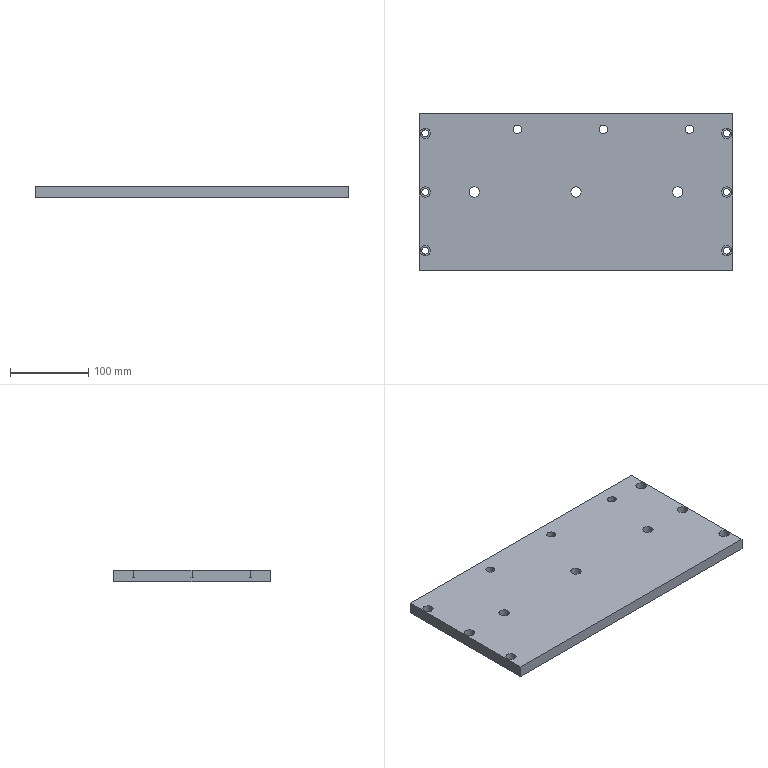Part | SolidWorks | features LPattern 4, Cut 2, ICE 2, MirrorPattern 2, Extrusion 1 | 1 solid | 48 faces | box 400 x 200 x 15 mm | volume 1180293 mm3 | cylinder 36 | plane 12 | commonest cylinder face diameters 13 x18 9 x12 11 x6
STEP:
#1=CARTESIAN_POINT('',(139.5,80.,0.));
#2=VERTEX_POINT('',#1);
#3=CARTESIAN_POINT('',(150.5,80.,0.));
#4=VERTEX_POINT('',#3);
#5=CARTESIAN_POINT('',(145.,80.,0.));
#6=DIRECTION('',(0.,0.,1.));
#7=DIRECTION('',(1.,0.,0.));
#8=AXIS2_PLACEMENT_3D('',#5,#6,#7);
#9=CIRCLE('',#8,5.5);
#10=EDGE_CURVE('',#2,#4,#9,.T.);
#11=ORIENTED_EDGE('',*,*,#10,.F.);
#12=CARTESIAN_POINT('',(139.5,80.,15.));
#13=VERTEX_POINT('',#12);
#14=CARTESIAN_POINT('',(139.5,80.,-36.));
#15=DIRECTION('',(0.,0.,1.));
#16=VECTOR('',#15,1000.);
#17=LINE('',#14,#16);
#18=EDGE_CURVE('',#2,#13,#17,.T.);
#19=ORIENTED_EDGE('',*,*,#18,.T.);
#20=CARTESIAN_POINT('',(150.5,80.,15.));
#21=VERTEX_POINT('',#20);
#22=CARTESIAN_POINT('',(145.,80.,15.));
#23=DIRECTION('',(0.,0.,1.));
#24=DIRECTION('',(1.,0.,0.));
#25=AXIS2_PLACEMENT_3D('',#22,#23,#24);
#26=CIRCLE('',#25,5.5);
#27=EDGE_CURVE('',#13,#21,#26,.T.);
#28=ORIENTED_EDGE('',*,*,#27,.T.);
#29=CARTESIAN_POINT('',(150.5,80.,-36.));
#30=DIRECTION('',(0.,0.,1.));
#31=VECTOR('',#30,1000.);
#32=LINE('',#29,#31);
#33=EDGE_CURVE('',#4,#21,#32,.T.);
#34=ORIENTED_EDGE('',*,*,#33,.F.);
#35=EDGE_LOOP('',(#11,#19,#28,#34));
#36=FACE_OUTER_BOUND('',#35,.T.);
#37=CARTESIAN_POINT('',(145.,80.,-36.));
#38=DIRECTION('',(0.,0.,1.));
#39=DIRECTION('',(1.,0.,0.));
#40=AXIS2_PLACEMENT_3D('',#37,#38,#39);
#41=CYLINDRICAL_SURFACE('',#40,5.5);
#42=ADVANCED_FACE('',(#36),#41,.F.);
#43=CARTESIAN_POINT('',(29.5,80.,0.));
#44=VERTEX_POINT('',#43);
#45=CARTESIAN_POINT('',(40.5,80.,0.));
#46=VERTEX_POINT('',#45);
#47=CARTESIAN_POINT('',(35.,80.,0.));
#48=DIRECTION('',(0.,0.,1.));
#49=DIRECTION('',(1.,0.,0.));
#50=AXIS2_PLACEMENT_3D('',#47,#48,#49);
#51=CIRCLE('',#50,5.5);
#52=EDGE_CURVE('',#44,#46,#51,.T.);
#53=ORIENTED_EDGE('',*,*,#52,.F.);
#54=CARTESIAN_POINT('',(29.5,80.,15.));
#55=VERTEX_POINT('',#54);
#56=CARTESIAN_POINT('',(29.5,80.,-36.));
#57=DIRECTION('',(0.,0.,1.));
#58=VECTOR('',#57,1000.);
#59=LINE('',#56,#58);
#60=EDGE_CURVE('',#44,#55,#59,.T.);
#61=ORIENTED_EDGE('',*,*,#60,.T.);
#62=CARTESIAN_POINT('',(40.5,80.,15.));
#63=VERTEX_POINT('',#62);
#64=CARTESIAN_POINT('',(35.,80.,15.));
#65=DIRECTION('',(0.,0.,1.));
#66=DIRECTION('',(1.,0.,0.));
#67=AXIS2_PLACEMENT_3D('',#64,#65,#66);
#68=CIRCLE('',#67,5.5);
#69=EDGE_CURVE('',#55,#63,#68,.T.);
#70=ORIENTED_EDGE('',*,*,#69,.T.);
#71=CARTESIAN_POINT('',(40.5,80.,-36.));
#72=DIRECTION('',(0.,0.,1.));
#73=VECTOR('',#72,1000.);
#74=LINE('',#71,#73);
#75=EDGE_CURVE('',#46,#63,#74,.T.);
#76=ORIENTED_EDGE('',*,*,#75,.F.);
#77=EDGE_LOOP('',(#53,#61,#70,#76));
#78=FACE_OUTER_BOUND('',#77,.T.);
#79=CARTESIAN_POINT('',(35.,80.,-36.));
#80=DIRECTION('',(0.,0.,1.));
#81=DIRECTION('',(1.,0.,0.));
#82=AXIS2_PLACEMENT_3D('',#79,#80,#81);
#83=CYLINDRICAL_SURFACE('',#82,5.5);
#84=ADVANCED_FACE('',(#78),#83,.F.);
#85=CARTESIAN_POINT('',(-80.5,80.,0.));
#86=VERTEX_POINT('',#85);
#87=CARTESIAN_POINT('',(-69.5,80.,0.));
#88=VERTEX_POINT('',#87);
#89=CARTESIAN_POINT('',(-75.,80.,0.));
#90=DIRECTION('',(0.,0.,1.));
#91=DIRECTION('',(1.,0.,0.));
#92=AXIS2_PLACEMENT_3D('',#89,#90,#91);
#93=CIRCLE('',#92,5.5);
#94=EDGE_CURVE('',#86,#88,#93,.T.);
#95=ORIENTED_EDGE('',*,*,#94,.F.);
#96=CARTESIAN_POINT('',(-80.5,80.,15.));
#97=VERTEX_POINT('',#96);
#98=CARTESIAN_POINT('',(-80.5,80.,-36.));
#99=DIRECTION('',(0.,0.,1.));
#100=VECTOR('',#99,1000.);
#101=LINE('',#98,#100);
#102=EDGE_CURVE('',#86,#97,#101,.T.);
#103=ORIENTED_EDGE('',*,*,#102,.T.);
#104=CARTESIAN_POINT('',(-69.5,80.,15.));
#105=VERTEX_POINT('',#104);
#106=CARTESIAN_POINT('',(-75.,80.,15.));
#107=DIRECTION('',(0.,0.,1.));
#108=DIRECTION('',(1.,0.,0.));
#109=AXIS2_PLACEMENT_3D('',#106,#107,#108);
#110=CIRCLE('',#109,5.5);
#111=EDGE_CURVE('',#97,#105,#110,.T.);
#112=ORIENTED_EDGE('',*,*,#111,.T.);
#113=CARTESIAN_POINT('',(-69.5,80.,-36.));
#114=DIRECTION('',(0.,0.,1.));
#115=VECTOR('',#114,1000.);
#116=LINE('',#113,#115);
#117=EDGE_CURVE('',#88,#105,#116,.T.);
#118=ORIENTED_EDGE('',*,*,#117,.F.);
#119=EDGE_LOOP('',(#95,#103,#112,#118));
#120=FACE_OUTER_BOUND('',#119,.T.);
#121=CARTESIAN_POINT('',(-75.,80.,-36.));
#122=DIRECTION('',(0.,0.,1.));
#123=DIRECTION('',(1.,0.,0.));
#124=AXIS2_PLACEMENT_3D('',#121,#122,#123);
#125=CYLINDRICAL_SURFACE('',#124,5.5);
#126=ADVANCED_FACE('',(#120),#125,.F.);
#127=CARTESIAN_POINT('',(123.5,0.,0.));
#128=VERTEX_POINT('',#127);
#129=CARTESIAN_POINT('',(136.5,0.,0.));
#130=VERTEX_POINT('',#129);
#131=CARTESIAN_POINT('',(130.,0.,0.));
#132=DIRECTION('',(0.,0.,1.));
#133=DIRECTION('',(1.,0.,0.));
#134=AXIS2_PLACEMENT_3D('',#131,#132,#133);
#135=CIRCLE('',#134,6.5);
#136=EDGE_CURVE('',#128,#130,#135,.T.);
#137=ORIENTED_EDGE('',*,*,#136,.F.);
#138=CARTESIAN_POINT('',(123.5,0.,15.));
#139=VERTEX_POINT('',#138);
#140=CARTESIAN_POINT('',(123.5,0.,-70.));
#141=DIRECTION('',(0.,0.,1.));
#142=VECTOR('',#141,1000.);
#143=LINE('',#140,#142);
#144=EDGE_CURVE('',#128,#139,#143,.T.);
#145=ORIENTED_EDGE('',*,*,#144,.T.);
#146=CARTESIAN_POINT('',(136.5,0.,15.));
#147=VERTEX_POINT('',#146);
#148=CARTESIAN_POINT('',(130.,0.,15.));
#149=DIRECTION('',(0.,0.,1.));
#150=DIRECTION('',(1.,0.,0.));
#151=AXIS2_PLACEMENT_3D('',#148,#149,#150);
#152=CIRCLE('',#151,6.5);
#153=EDGE_CURVE('',#139,#147,#152,.T.);
#154=ORIENTED_EDGE('',*,*,#153,.T.);
#155=CARTESIAN_POINT('',(136.5,0.,-70.));
#156=DIRECTION('',(0.,0.,1.));
#157=VECTOR('',#156,1000.);
#158=LINE('',#155,#157);
#159=EDGE_CURVE('',#130,#147,#158,.T.);
#160=ORIENTED_EDGE('',*,*,#159,.F.);
#161=EDGE_LOOP('',(#137,#145,#154,#160));
#162=FACE_OUTER_BOUND('',#161,.T.);
#163=CARTESIAN_POINT('',(130.,0.,-70.));
#164=DIRECTION('',(0.,0.,1.));
#165=DIRECTION('',(1.,0.,0.));
#166=AXIS2_PLACEMENT_3D('',#163,#164,#165);
#167=CYLINDRICAL_SURFACE('',#166,6.5);
#168=ADVANCED_FACE('',(#162),#167,.F.);
#169=CARTESIAN_POINT('',(-6.5,0.,0.));
#170=VERTEX_POINT('',#169);
#171=CARTESIAN_POINT('',(6.5,0.,0.));
#172=VERTEX_POINT('',#171);
#173=CARTESIAN_POINT('',(0.,0.,0.));
#174=DIRECTION('',(0.,0.,1.));
#175=DIRECTION('',(1.,0.,0.));
#176=AXIS2_PLACEMENT_3D('',#173,#174,#175);
#177=CIRCLE('',#176,6.5);
#178=EDGE_CURVE('',#170,#172,#177,.T.);
#179=ORIENTED_EDGE('',*,*,#178,.F.);
#180=CARTESIAN_POINT('',(-6.5,0.,15.));
#181=VERTEX_POINT('',#180);
#182=CARTESIAN_POINT('',(-6.5,0.,-70.));
#183=DIRECTION('',(0.,0.,1.));
#184=VECTOR('',#183,1000.);
#185=LINE('',#182,#184);
#186=EDGE_CURVE('',#170,#181,#185,.T.);
#187=ORIENTED_EDGE('',*,*,#186,.T.);
#188=CARTESIAN_POINT('',(6.5,0.,15.));
#189=VERTEX_POINT('',#188);
#190=CARTESIAN_POINT('',(0.,0.,15.));
#191=DIRECTION('',(0.,0.,1.));
#192=DIRECTION('',(1.,0.,0.));
#193=AXIS2_PLACEMENT_3D('',#190,#191,#192);
#194=CIRCLE('',#193,6.5);
#195=EDGE_CURVE('',#181,#189,#194,.T.);
#196=ORIENTED_EDGE('',*,*,#195,.T.);
#197=CARTESIAN_POINT('',(6.5,0.,-70.));
#198=DIRECTION('',(0.,0.,1.));
#199=VECTOR('',#198,1000.);
#200=LINE('',#197,#199);
#201=EDGE_CURVE('',#172,#189,#200,.T.);
#202=ORIENTED_EDGE('',*,*,#201,.F.);
#203=EDGE_LOOP('',(#179,#187,#196,#202));
#204=FACE_OUTER_BOUND('',#203,.T.);
#205=CARTESIAN_POINT('',(0.,0.,-70.));
#206=DIRECTION('',(0.,0.,1.));
#207=DIRECTION('',(1.,0.,0.));
#208=AXIS2_PLACEMENT_3D('',#205,#206,#207);
#209=CYLINDRICAL_SURFACE('',#208,6.5);
#210=ADVANCED_FACE('',(#204),#209,.F.);
#211=CARTESIAN_POINT('',(-136.5,0.,0.));
#212=VERTEX_POINT('',#211);
#213=CARTESIAN_POINT('',(-123.5,0.,0.));
#214=VERTEX_POINT('',#213);
#215=CARTESIAN_POINT('',(-130.,0.,0.));
#216=DIRECTION('',(0.,0.,1.));
#217=DIRECTION('',(1.,0.,0.));
#218=AXIS2_PLACEMENT_3D('',#215,#216,#217);
#219=CIRCLE('',#218,6.5);
#220=EDGE_CURVE('',#212,#214,#219,.T.);
#221=ORIENTED_EDGE('',*,*,#220,.F.);
#222=CARTESIAN_POINT('',(-136.5,0.,15.));
#223=VERTEX_POINT('',#222);
#224=CARTESIAN_POINT('',(-136.5,0.,-70.));
#225=DIRECTION('',(0.,0.,1.));
#226=VECTOR('',#225,1000.);
#227=LINE('',#224,#226);
#228=EDGE_CURVE('',#212,#223,#227,.T.);
#229=ORIENTED_EDGE('',*,*,#228,.T.);
#230=CARTESIAN_POINT('',(-123.5,0.,15.));
#231=VERTEX_POINT('',#230);
#232=CARTESIAN_POINT('',(-130.,0.,15.));
#233=DIRECTION('',(0.,0.,1.));
#234=DIRECTION('',(1.,0.,0.));
#235=AXIS2_PLACEMENT_3D('',#232,#233,#234);
#236=CIRCLE('',#235,6.5);
#237=EDGE_CURVE('',#223,#231,#236,.T.);
#238=ORIENTED_EDGE('',*,*,#237,.T.);
#239=CARTESIAN_POINT('',(-123.5,0.,-70.));
#240=DIRECTION('',(0.,0.,1.));
#241=VECTOR('',#240,1000.);
#242=LINE('',#239,#241);
#243=EDGE_CURVE('',#214,#231,#242,.T.);
#244=ORIENTED_EDGE('',*,*,#243,.F.);
#245=EDGE_LOOP('',(#221,#229,#238,#244));
#246=FACE_OUTER_BOUND('',#245,.T.);
#247=CARTESIAN_POINT('',(-130.,0.,-70.));
#248=DIRECTION('',(0.,0.,1.));
#249=DIRECTION('',(1.,0.,0.));
#250=AXIS2_PLACEMENT_3D('',#247,#248,#249);
#251=CYLINDRICAL_SURFACE('',#250,6.5);
#252=ADVANCED_FACE('',(#246),#251,.F.);
#253=CARTESIAN_POINT('',(197.,-75.,0.));
#254=VERTEX_POINT('',#253);
#255=CARTESIAN_POINT('',(188.,-75.,0.));
#256=VERTEX_POINT('',#255);
#257=CARTESIAN_POINT('',(192.5,-75.,0.));
#258=DIRECTION('',(0.,0.,-1.));
#259=DIRECTION('',(1.,0.,0.));
#260=AXIS2_PLACEMENT_3D('',#257,#258,#259);
#261=CIRCLE('',#260,4.5);
#262=EDGE_CURVE('',#254,#256,#261,.T.);
#263=ORIENTED_EDGE('',*,*,#262,.T.);
#264=CARTESIAN_POINT('',(188.,-75.,6.));
#265=VERTEX_POINT('',#264);
#266=CARTESIAN_POINT('',(188.,-75.,-70.));
#267=DIRECTION('',(0.,0.,1.));
#268=VECTOR('',#267,1000.);
#269=LINE('',#266,#268);
#270=EDGE_CURVE('',#256,#265,#269,.T.);
#271=ORIENTED_EDGE('',*,*,#270,.T.);
#272=CARTESIAN_POINT('',(197.,-75.,6.));
#273=VERTEX_POINT('',#272);
#274=CARTESIAN_POINT('',(192.5,-75.,6.));
#275=DIRECTION('',(0.,0.,-1.));
#276=DIRECTION('',(1.,0.,0.));
#277=AXIS2_PLACEMENT_3D('',#274,#275,#276);
#278=CIRCLE('',#277,4.5);
#279=EDGE_CURVE('',#273,#265,#278,.T.);
#280=ORIENTED_EDGE('',*,*,#279,.F.);
#281=CARTESIAN_POINT('',(197.,-75.,-70.));
#282=DIRECTION('',(0.,0.,1.));
#283=VECTOR('',#282,1000.);
#284=LINE('',#281,#283);
#285=EDGE_CURVE('',#254,#273,#284,.T.);
#286=ORIENTED_EDGE('',*,*,#285,.F.);
#287=EDGE_LOOP('',(#263,#271,#280,#286));
#288=FACE_OUTER_BOUND('',#287,.T.);
#289=CARTESIAN_POINT('',(192.5,-75.,-70.));
#290=DIRECTION('',(0.,0.,1.));
#291=DIRECTION('',(1.,0.,0.));
#292=AXIS2_PLACEMENT_3D('',#289,#290,#291);
#293=CYLINDRICAL_SURFACE('',#292,4.5);
#294=ADVANCED_FACE('',(#288),#293,.F.);
#295=CARTESIAN_POINT('',(197.,0.,0.));
#296=VERTEX_POINT('',#295);
#297=CARTESIAN_POINT('',(188.,0.,0.));
#298=VERTEX_POINT('',#297);
#299=CARTESIAN_POINT('',(192.5,0.,0.));
#300=DIRECTION('',(0.,0.,-1.));
#301=DIRECTION('',(1.,0.,0.));
#302=AXIS2_PLACEMENT_3D('',#299,#300,#301);
#303=CIRCLE('',#302,4.5);
#304=EDGE_CURVE('',#296,#298,#303,.T.);
#305=ORIENTED_EDGE('',*,*,#304,.T.);
#306=CARTESIAN_POINT('',(188.,0.,6.));
#307=VERTEX_POINT('',#306);
#308=CARTESIAN_POINT('',(188.,0.,-70.));
#309=DIRECTION('',(0.,0.,1.));
#310=VECTOR('',#309,1000.);
#311=LINE('',#308,#310);
#312=EDGE_CURVE('',#298,#307,#311,.T.);
#313=ORIENTED_EDGE('',*,*,#312,.T.);
#314=CARTESIAN_POINT('',(197.,0.,6.));
#315=VERTEX_POINT('',#314);
#316=CARTESIAN_POINT('',(192.5,0.,6.));
#317=DIRECTION('',(0.,0.,-1.));
#318=DIRECTION('',(1.,0.,0.));
#319=AXIS2_PLACEMENT_3D('',#316,#317,#318);
#320=CIRCLE('',#319,4.5);
#321=EDGE_CURVE('',#315,#307,#320,.T.);
#322=ORIENTED_EDGE('',*,*,#321,.F.);
#323=CARTESIAN_POINT('',(197.,0.,-70.));
#324=DIRECTION('',(0.,0.,1.));
#325=VECTOR('',#324,1000.);
#326=LINE('',#323,#325);
#327=EDGE_CURVE('',#296,#315,#326,.T.);
#328=ORIENTED_EDGE('',*,*,#327,.F.);
#329=EDGE_LOOP('',(#305,#313,#322,#328));
#330=FACE_OUTER_BOUND('',#329,.T.);
#331=CARTESIAN_POINT('',(192.5,0.,-70.));
#332=DIRECTION('',(0.,0.,1.));
#333=DIRECTION('',(1.,0.,0.));
#334=AXIS2_PLACEMENT_3D('',#331,#332,#333);
#335=CYLINDRICAL_SURFACE('',#334,4.5);
#336=ADVANCED_FACE('',(#330),#335,.F.);
#337=CARTESIAN_POINT('',(197.,75.,0.));
#338=VERTEX_POINT('',#337);
#339=CARTESIAN_POINT('',(188.,75.,0.));
#340=VERTEX_POINT('',#339);
#341=CARTESIAN_POINT('',(192.5,75.,0.));
#342=DIRECTION('',(0.,0.,-1.));
#343=DIRECTION('',(1.,0.,0.));
#344=AXIS2_PLACEMENT_3D('',#341,#342,#343);
#345=CIRCLE('',#344,4.5);
#346=EDGE_CURVE('',#338,#340,#345,.T.);
#347=ORIENTED_EDGE('',*,*,#346,.T.);
#348=CARTESIAN_POINT('',(188.,75.,6.));
#349=VERTEX_POINT('',#348);
#350=CARTESIAN_POINT('',(188.,75.,-70.));
#351=DIRECTION('',(0.,0.,1.));
#352=VECTOR('',#351,1000.);
#353=LINE('',#350,#352);
#354=EDGE_CURVE('',#340,#349,#353,.T.);
#355=ORIENTED_EDGE('',*,*,#354,.T.);
#356=CARTESIAN_POINT('',(197.,75.,6.));
#357=VERTEX_POINT('',#356);
#358=CARTESIAN_POINT('',(192.5,75.,6.));
#359=DIRECTION('',(0.,0.,-1.));
#360=DIRECTION('',(1.,0.,0.));
#361=AXIS2_PLACEMENT_3D('',#358,#359,#360);
#362=CIRCLE('',#361,4.5);
#363=EDGE_CURVE('',#357,#349,#362,.T.);
#364=ORIENTED_EDGE('',*,*,#363,.F.);
#365=CARTESIAN_POINT('',(197.,75.,-70.));
#366=DIRECTION('',(0.,0.,1.));
#367=VECTOR('',#366,1000.);
#368=LINE('',#365,#367);
#369=EDGE_CURVE('',#338,#357,#368,.T.);
#370=ORIENTED_EDGE('',*,*,#369,.F.);
#371=EDGE_LOOP('',(#347,#355,#364,#370));
#372=FACE_OUTER_BOUND('',#371,.T.);
#373=CARTESIAN_POINT('',(192.5,75.,-70.));
#374=DIRECTION('',(0.,0.,1.));
#375=DIRECTION('',(1.,0.,0.));
#376=AXIS2_PLACEMENT_3D('',#373,#374,#375);
#377=CYLINDRICAL_SURFACE('',#376,4.5);
#378=ADVANCED_FACE('',(#372),#377,.F.);
#379=CARTESIAN_POINT('',(-197.,-75.,0.));
#380=VERTEX_POINT('',#379);
#381=CARTESIAN_POINT('',(-188.,-75.,0.));
#382=VERTEX_POINT('',#381);
#383=CARTESIAN_POINT('',(-192.5,-75.,0.));
#384=DIRECTION('',(0.,0.,1.));
#385=DIRECTION('',(1.,0.,0.));
#386=AXIS2_PLACEMENT_3D('',#383,#384,#385);
#387=CIRCLE('',#386,4.5);
#388=EDGE_CURVE('',#380,#382,#387,.T.);
#389=ORIENTED_EDGE('',*,*,#388,.F.);
#390=CARTESIAN_POINT('',(-197.,-75.,6.));
#391=VERTEX_POINT('',#390);
#392=CARTESIAN_POINT('',(-197.,-75.,-70.));
#393=DIRECTION('',(0.,0.,1.));
#394=VECTOR('',#393,1000.);
#395=LINE('',#392,#394);
#396=EDGE_CURVE('',#380,#391,#395,.T.);
#397=ORIENTED_EDGE('',*,*,#396,.T.);
#398=CARTESIAN_POINT('',(-188.,-75.,6.));
#399=VERTEX_POINT('',#398);
#400=CARTESIAN_POINT('',(-192.5,-75.,6.));
#401=DIRECTION('',(0.,0.,1.));
#402=DIRECTION('',(1.,0.,0.));
#403=AXIS2_PLACEMENT_3D('',#400,#401,#402);
#404=CIRCLE('',#403,4.5);
#405=EDGE_CURVE('',#391,#399,#404,.T.);
#406=ORIENTED_EDGE('',*,*,#405,.T.);
#407=CARTESIAN_POINT('',(-188.,-75.,-70.));
#408=DIRECTION('',(0.,0.,1.));
#409=VECTOR('',#408,1000.);
#410=LINE('',#407,#409);
#411=EDGE_CURVE('',#382,#399,#410,.T.);
#412=ORIENTED_EDGE('',*,*,#411,.F.);
#413=EDGE_LOOP('',(#389,#397,#406,#412));
#414=FACE_OUTER_BOUND('',#413,.T.);
#415=CARTESIAN_POINT('',(-192.5,-75.,-70.));
#416=DIRECTION('',(0.,0.,1.));
#417=DIRECTION('',(1.,0.,0.));
#418=AXIS2_PLACEMENT_3D('',#415,#416,#417);
#419=CYLINDRICAL_SURFACE('',#418,4.5);
#420=ADVANCED_FACE('',(#414),#419,.F.);
#421=CARTESIAN_POINT('',(-197.,0.,0.));
#422=VERTEX_POINT('',#421);
#423=CARTESIAN_POINT('',(-188.,0.,0.));
#424=VERTEX_POINT('',#423);
#425=CARTESIAN_POINT('',(-192.5,0.,0.));
#426=DIRECTION('',(0.,0.,1.));
#427=DIRECTION('',(1.,0.,0.));
#428=AXIS2_PLACEMENT_3D('',#425,#426,#427);
#429=CIRCLE('',#428,4.5);
#430=EDGE_CURVE('',#422,#424,#429,.T.);
#431=ORIENTED_EDGE('',*,*,#430,.F.);
#432=CARTESIAN_POINT('',(-197.,0.,6.));
#433=VERTEX_POINT('',#432);
#434=CARTESIAN_POINT('',(-197.,0.,-70.));
#435=DIRECTION('',(0.,0.,1.));
#436=VECTOR('',#435,1000.);
#437=LINE('',#434,#436);
#438=EDGE_CURVE('',#422,#433,#437,.T.);
#439=ORIENTED_EDGE('',*,*,#438,.T.);
#440=CARTESIAN_POINT('',(-188.,0.,6.));
#441=VERTEX_POINT('',#440);
#442=CARTESIAN_POINT('',(-192.5,0.,6.));
#443=DIRECTION('',(0.,0.,1.));
#444=DIRECTION('',(1.,0.,0.));
#445=AXIS2_PLACEMENT_3D('',#442,#443,#444);
#446=CIRCLE('',#445,4.5);
#447=EDGE_CURVE('',#433,#441,#446,.T.);
#448=ORIENTED_EDGE('',*,*,#447,.T.);
#449=CARTESIAN_POINT('',(-188.,0.,-70.));
#450=DIRECTION('',(0.,0.,1.));
#451=VECTOR('',#450,1000.);
#452=LINE('',#449,#451);
#453=EDGE_CURVE('',#424,#441,#452,.T.);
#454=ORIENTED_EDGE('',*,*,#453,.F.);
#455=EDGE_LOOP('',(#431,#439,#448,#454));
#456=FACE_OUTER_BOUND('',#455,.T.);
#457=CARTESIAN_POINT('',(-192.5,0.,-70.));
#458=DIRECTION('',(0.,0.,1.));
#459=DIRECTION('',(1.,0.,0.));
#460=AXIS2_PLACEMENT_3D('',#457,#458,#459);
#461=CYLINDRICAL_SURFACE('',#460,4.5);
#462=ADVANCED_FACE('',(#456),#461,.F.);
#463=CARTESIAN_POINT('',(-197.,75.,0.));
#464=VERTEX_POINT('',#463);
#465=CARTESIAN_POINT('',(-188.,75.,0.));
#466=VERTEX_POINT('',#465);
#467=CARTESIAN_POINT('',(-192.5,75.,0.));
#468=DIRECTION('',(0.,0.,1.));
#469=DIRECTION('',(1.,0.,0.));
#470=AXIS2_PLACEMENT_3D('',#467,#468,#469);
#471=CIRCLE('',#470,4.5);
#472=EDGE_CURVE('',#464,#466,#471,.T.);
#473=ORIENTED_EDGE('',*,*,#472,.F.);
#474=CARTESIAN_POINT('',(-197.,75.,6.));
#475=VERTEX_POINT('',#474);
#476=CARTESIAN_POINT('',(-197.,75.,-70.));
#477=DIRECTION('',(0.,0.,1.));
#478=VECTOR('',#477,1000.);
#479=LINE('',#476,#478);
#480=EDGE_CURVE('',#464,#475,#479,.T.);
#481=ORIENTED_EDGE('',*,*,#480,.T.);
#482=CARTESIAN_POINT('',(-188.,75.,6.));
#483=VERTEX_POINT('',#482);
#484=CARTESIAN_POINT('',(-192.5,75.,6.));
#485=DIRECTION('',(0.,0.,1.));
#486=DIRECTION('',(1.,0.,0.));
#487=AXIS2_PLACEMENT_3D('',#484,#485,#486);
#488=CIRCLE('',#487,4.5);
#489=EDGE_CURVE('',#475,#483,#488,.T.);
#490=ORIENTED_EDGE('',*,*,#489,.T.);
#491=CARTESIAN_POINT('',(-188.,75.,-70.));
#492=DIRECTION('',(0.,0.,1.));
#493=VECTOR('',#492,1000.);
#494=LINE('',#491,#493);
#495=EDGE_CURVE('',#466,#483,#494,.T.);
#496=ORIENTED_EDGE('',*,*,#495,.F.);
#497=EDGE_LOOP('',(#473,#481,#490,#496));
#498=FACE_OUTER_BOUND('',#497,.T.);
#499=CARTESIAN_POINT('',(-192.5,75.,-70.));
#500=DIRECTION('',(0.,0.,1.));
#501=DIRECTION('',(1.,0.,0.));
#502=AXIS2_PLACEMENT_3D('',#499,#500,#501);
#503=CYLINDRICAL_SURFACE('',#502,4.5);
#504=ADVANCED_FACE('',(#498),#503,.F.);
#505=CARTESIAN_POINT('',(199.,-75.,6.));
#506=VERTEX_POINT('',#505);
#507=CARTESIAN_POINT('',(186.,-75.,6.));
#508=VERTEX_POINT('',#507);
#509=CARTESIAN_POINT('',(192.5,-75.,6.));
#510=DIRECTION('',(0.,0.,-1.));
#511=DIRECTION('',(-1.,0.,0.));
#512=AXIS2_PLACEMENT_3D('',#509,#510,#511);
#513=CIRCLE('',#512,6.5);
#514=EDGE_CURVE('',#506,#508,#513,.T.);
#515=ORIENTED_EDGE('',*,*,#514,.T.);
#516=CARTESIAN_POINT('',(186.,-75.,15.));
#517=VERTEX_POINT('',#516);
#518=CARTESIAN_POINT('',(186.,-75.,6.));
#519=DIRECTION('',(0.,0.,1.));
#520=VECTOR('',#519,1000.);
#521=LINE('',#518,#520);
#522=EDGE_CURVE('',#508,#517,#521,.T.);
#523=ORIENTED_EDGE('',*,*,#522,.T.);
#524=CARTESIAN_POINT('',(199.,-75.,15.));
#525=VERTEX_POINT('',#524);
#526=CARTESIAN_POINT('',(192.5,-75.,15.));
#527=DIRECTION('',(0.,0.,-1.));
#528=DIRECTION('',(-1.,0.,0.));
#529=AXIS2_PLACEMENT_3D('',#526,#527,#528);
#530=CIRCLE('',#529,6.5);
#531=EDGE_CURVE('',#525,#517,#530,.T.);
#532=ORIENTED_EDGE('',*,*,#531,.F.);
#533=CARTESIAN_POINT('',(199.,-75.,6.));
#534=DIRECTION('',(0.,0.,1.));
#535=VECTOR('',#534,1000.);
#536=LINE('',#533,#535);
#537=EDGE_CURVE('',#506,#525,#536,.T.);
#538=ORIENTED_EDGE('',*,*,#537,.F.);
#539=EDGE_LOOP('',(#515,#523,#532,#538));
#540=FACE_OUTER_BOUND('',#539,.T.);
#541=CARTESIAN_POINT('',(192.5,-75.,6.));
#542=DIRECTION('',(0.,0.,1.));
#543=DIRECTION('',(1.,0.,0.));
#544=AXIS2_PLACEMENT_3D('',#541,#542,#543);
#545=CYLINDRICAL_SURFACE('',#544,6.5);
#546=ADVANCED_FACE('',(#540),#545,.F.);
#547=CARTESIAN_POINT('',(199.,0.,6.));
#548=VERTEX_POINT('',#547);
#549=CARTESIAN_POINT('',(186.,0.,6.));
#550=VERTEX_POINT('',#549);
#551=CARTESIAN_POINT('',(192.5,0.,6.));
#552=DIRECTION('',(0.,0.,-1.));
#553=DIRECTION('',(-1.,0.,0.));
#554=AXIS2_PLACEMENT_3D('',#551,#552,#553);
#555=CIRCLE('',#554,6.5);
#556=EDGE_CURVE('',#548,#550,#555,.T.);
#557=ORIENTED_EDGE('',*,*,#556,.T.);
#558=CARTESIAN_POINT('',(186.,0.,15.));
#559=VERTEX_POINT('',#558);
#560=CARTESIAN_POINT('',(186.,0.,6.));
#561=DIRECTION('',(0.,0.,1.));
#562=VECTOR('',#561,1000.);
#563=LINE('',#560,#562);
#564=EDGE_CURVE('',#550,#559,#563,.T.);
#565=ORIENTED_EDGE('',*,*,#564,.T.);
#566=CARTESIAN_POINT('',(199.,0.,15.));
#567=VERTEX_POINT('',#566);
#568=CARTESIAN_POINT('',(192.5,0.,15.));
#569=DIRECTION('',(0.,0.,-1.));
#570=DIRECTION('',(-1.,0.,0.));
#571=AXIS2_PLACEMENT_3D('',#568,#569,#570);
#572=CIRCLE('',#571,6.5);
#573=EDGE_CURVE('',#567,#559,#572,.T.);
#574=ORIENTED_EDGE('',*,*,#573,.F.);
#575=CARTESIAN_POINT('',(199.,0.,6.));
#576=DIRECTION('',(0.,0.,1.));
#577=VECTOR('',#576,1000.);
#578=LINE('',#575,#577);
#579=EDGE_CURVE('',#548,#567,#578,.T.);
#580=ORIENTED_EDGE('',*,*,#579,.F.);
#581=EDGE_LOOP('',(#557,#565,#574,#580));
#582=FACE_OUTER_BOUND('',#581,.T.);
#583=CARTESIAN_POINT('',(192.5,0.,6.));
#584=DIRECTION('',(0.,0.,1.));
#585=DIRECTION('',(1.,0.,0.));
#586=AXIS2_PLACEMENT_3D('',#583,#584,#585);
#587=CYLINDRICAL_SURFACE('',#586,6.5);
#588=ADVANCED_FACE('',(#582),#587,.F.);
#589=CARTESIAN_POINT('',(199.,75.,6.));
#590=VERTEX_POINT('',#589);
#591=CARTESIAN_POINT('',(186.,75.,6.));
#592=VERTEX_POINT('',#591);
#593=CARTESIAN_POINT('',(192.5,75.,6.));
#594=DIRECTION('',(0.,0.,-1.));
#595=DIRECTION('',(-1.,0.,0.));
#596=AXIS2_PLACEMENT_3D('',#593,#594,#595);
#597=CIRCLE('',#596,6.5);
#598=EDGE_CURVE('',#590,#592,#597,.T.);
#599=ORIENTED_EDGE('',*,*,#598,.T.);
#600=CARTESIAN_POINT('',(186.,75.,15.));
#601=VERTEX_POINT('',#600);
#602=CARTESIAN_POINT('',(186.,75.,6.));
#603=DIRECTION('',(0.,0.,1.));
#604=VECTOR('',#603,1000.);
#605=LINE('',#602,#604);
#606=EDGE_CURVE('',#592,#601,#605,.T.);
#607=ORIENTED_EDGE('',*,*,#606,.T.);
#608=CARTESIAN_POINT('',(199.,75.,15.));
#609=VERTEX_POINT('',#608);
#610=CARTESIAN_POINT('',(192.5,75.,15.));
#611=DIRECTION('',(0.,0.,-1.));
#612=DIRECTION('',(-1.,0.,0.));
#613=AXIS2_PLACEMENT_3D('',#610,#611,#612);
#614=CIRCLE('',#613,6.5);
#615=EDGE_CURVE('',#609,#601,#614,.T.);
#616=ORIENTED_EDGE('',*,*,#615,.F.);
#617=CARTESIAN_POINT('',(199.,75.,6.));
#618=DIRECTION('',(0.,0.,1.));
#619=VECTOR('',#618,1000.);
#620=LINE('',#617,#619);
#621=EDGE_CURVE('',#590,#609,#620,.T.);
#622=ORIENTED_EDGE('',*,*,#621,.F.);
#623=EDGE_LOOP('',(#599,#607,#616,#622));
#624=FACE_OUTER_BOUND('',#623,.T.);
#625=CARTESIAN_POINT('',(192.5,75.,6.));
#626=DIRECTION('',(0.,0.,1.));
#627=DIRECTION('',(1.,0.,0.));
#628=AXIS2_PLACEMENT_3D('',#625,#626,#627);
#629=CYLINDRICAL_SURFACE('',#628,6.5);
#630=ADVANCED_FACE('',(#624),#629,.F.);
#631=CARTESIAN_POINT('',(-199.,-75.,6.));
#632=VERTEX_POINT('',#631);
#633=CARTESIAN_POINT('',(-186.,-75.,6.));
#634=VERTEX_POINT('',#633);
#635=CARTESIAN_POINT('',(-192.5,-75.,6.));
#636=DIRECTION('',(0.,0.,1.));
#637=DIRECTION('',(1.,0.,0.));
#638=AXIS2_PLACEMENT_3D('',#635,#636,#637);
#639=CIRCLE('',#638,6.5);
#640=EDGE_CURVE('',#632,#634,#639,.T.);
#641=ORIENTED_EDGE('',*,*,#640,.F.);
#642=CARTESIAN_POINT('',(-199.,-75.,15.));
#643=VERTEX_POINT('',#642);
#644=CARTESIAN_POINT('',(-199.,-75.,6.));
#645=DIRECTION('',(0.,0.,1.));
#646=VECTOR('',#645,1000.);
#647=LINE('',#644,#646);
#648=EDGE_CURVE('',#632,#643,#647,.T.);
#649=ORIENTED_EDGE('',*,*,#648,.T.);
#650=CARTESIAN_POINT('',(-186.,-75.,15.));
#651=VERTEX_POINT('',#650);
#652=CARTESIAN_POINT('',(-192.5,-75.,15.));
#653=DIRECTION('',(0.,0.,1.));
#654=DIRECTION('',(1.,0.,0.));
#655=AXIS2_PLACEMENT_3D('',#652,#653,#654);
#656=CIRCLE('',#655,6.5);
#657=EDGE_CURVE('',#643,#651,#656,.T.);
#658=ORIENTED_EDGE('',*,*,#657,.T.);
#659=CARTESIAN_POINT('',(-186.,-75.,6.));
#660=DIRECTION('',(0.,0.,1.));
#661=VECTOR('',#660,1000.);
#662=LINE('',#659,#661);
#663=EDGE_CURVE('',#634,#651,#662,.T.);
#664=ORIENTED_EDGE('',*,*,#663,.F.);
#665=EDGE_LOOP('',(#641,#649,#658,#664));
#666=FACE_OUTER_BOUND('',#665,.T.);
#667=CARTESIAN_POINT('',(-192.5,-75.,6.));
#668=DIRECTION('',(0.,0.,1.));
#669=DIRECTION('',(1.,0.,0.));
#670=AXIS2_PLACEMENT_3D('',#667,#668,#669);
#671=CYLINDRICAL_SURFACE('',#670,6.5);
#672=ADVANCED_FACE('',(#666),#671,.F.);
#673=CARTESIAN_POINT('',(-199.,0.,6.));
#674=VERTEX_POINT('',#673);
#675=CARTESIAN_POINT('',(-186.,0.,6.));
#676=VERTEX_POINT('',#675);
#677=CARTESIAN_POINT('',(-192.5,0.,6.));
#678=DIRECTION('',(0.,0.,1.));
#679=DIRECTION('',(1.,0.,0.));
#680=AXIS2_PLACEMENT_3D('',#677,#678,#679);
#681=CIRCLE('',#680,6.5);
#682=EDGE_CURVE('',#674,#676,#681,.T.);
#683=ORIENTED_EDGE('',*,*,#682,.F.);
#684=CARTESIAN_POINT('',(-199.,0.,15.));
#685=VERTEX_POINT('',#684);
#686=CARTESIAN_POINT('',(-199.,0.,6.));
#687=DIRECTION('',(0.,0.,1.));
#688=VECTOR('',#687,1000.);
#689=LINE('',#686,#688);
#690=EDGE_CURVE('',#674,#685,#689,.T.);
#691=ORIENTED_EDGE('',*,*,#690,.T.);
#692=CARTESIAN_POINT('',(-186.,0.,15.));
#693=VERTEX_POINT('',#692);
#694=CARTESIAN_POINT('',(-192.5,0.,15.));
#695=DIRECTION('',(0.,0.,1.));
#696=DIRECTION('',(1.,0.,0.));
#697=AXIS2_PLACEMENT_3D('',#694,#695,#696);
#698=CIRCLE('',#697,6.5);
#699=EDGE_CURVE('',#685,#693,#698,.T.);
#700=ORIENTED_EDGE('',*,*,#699,.T.);
#701=CARTESIAN_POINT('',(-186.,0.,6.));
#702=DIRECTION('',(0.,0.,1.));
#703=VECTOR('',#702,1000.);
#704=LINE('',#701,#703);
#705=EDGE_CURVE('',#676,#693,#704,.T.);
#706=ORIENTED_EDGE('',*,*,#705,.F.);
#707=EDGE_LOOP('',(#683,#691,#700,#706));
#708=FACE_OUTER_BOUND('',#707,.T.);
#709=CARTESIAN_POINT('',(-192.5,0.,6.));
#710=DIRECTION('',(0.,0.,1.));
#711=DIRECTION('',(1.,0.,0.));
#712=AXIS2_PLACEMENT_3D('',#709,#710,#711);
#713=CYLINDRICAL_SURFACE('',#712,6.5);
#714=ADVANCED_FACE('',(#708),#713,.F.);
#715=CARTESIAN_POINT('',(-199.,75.,6.));
#716=VERTEX_POINT('',#715);
#717=CARTESIAN_POINT('',(-186.,75.,6.));
#718=VERTEX_POINT('',#717);
#719=CARTESIAN_POINT('',(-192.5,75.,6.));
#720=DIRECTION('',(0.,0.,1.));
#721=DIRECTION('',(1.,0.,0.));
#722=AXIS2_PLACEMENT_3D('',#719,#720,#721);
#723=CIRCLE('',#722,6.5);
#724=EDGE_CURVE('',#716,#718,#723,.T.);
#725=ORIENTED_EDGE('',*,*,#724,.F.);
#726=CARTESIAN_POINT('',(-199.,75.,15.));
#727=VERTEX_POINT('',#726);
#728=CARTESIAN_POINT('',(-199.,75.,6.));
#729=DIRECTION('',(0.,0.,1.));
#730=VECTOR('',#729,1000.);
#731=LINE('',#728,#730);
#732=EDGE_CURVE('',#716,#727,#731,.T.);
#733=ORIENTED_EDGE('',*,*,#732,.T.);
#734=CARTESIAN_POINT('',(-186.,75.,15.));
#735=VERTEX_POINT('',#734);
#736=CARTESIAN_POINT('',(-192.5,75.,15.));
#737=DIRECTION('',(0.,0.,1.));
#738=DIRECTION('',(1.,0.,0.));
#739=AXIS2_PLACEMENT_3D('',#736,#737,#738);
#740=CIRCLE('',#739,6.5);
#741=EDGE_CURVE('',#727,#735,#740,.T.);
#742=ORIENTED_EDGE('',*,*,#741,.T.);
#743=CARTESIAN_POINT('',(-186.,75.,6.));
#744=DIRECTION('',(0.,0.,1.));
#745=VECTOR('',#744,1000.);
#746=LINE('',#743,#745);
#747=EDGE_CURVE('',#718,#735,#746,.T.);
#748=ORIENTED_EDGE('',*,*,#747,.F.);
#749=EDGE_LOOP('',(#725,#733,#742,#748));
#750=FACE_OUTER_BOUND('',#749,.T.);
#751=CARTESIAN_POINT('',(-192.5,75.,6.));
#752=DIRECTION('',(0.,0.,1.));
#753=DIRECTION('',(1.,0.,0.));
#754=AXIS2_PLACEMENT_3D('',#751,#752,#753);
#755=CYLINDRICAL_SURFACE('',#754,6.5);
#756=ADVANCED_FACE('',(#750),#755,.F.);
#757=CARTESIAN_POINT('',(35.,80.,0.));
#758=DIRECTION('',(0.,0.,1.));
#759=DIRECTION('',(1.,0.,0.));
#760=AXIS2_PLACEMENT_3D('',#757,#758,#759);
#761=CIRCLE('',#760,5.5);
#762=EDGE_CURVE('',#46,#44,#761,.T.);
#763=ORIENTED_EDGE('',*,*,#762,.T.);
#764=ORIENTED_EDGE('',*,*,#52,.T.);
#765=EDGE_LOOP('',(#763,#764));
#766=FACE_BOUND('',#765,.T.);
#767=CARTESIAN_POINT('',(-75.,80.,0.));
#768=DIRECTION('',(0.,0.,1.));
#769=DIRECTION('',(1.,0.,0.));
#770=AXIS2_PLACEMENT_3D('',#767,#768,#769);
#771=CIRCLE('',#770,5.5);
#772=EDGE_CURVE('',#88,#86,#771,.T.);
#773=ORIENTED_EDGE('',*,*,#772,.T.);
#774=ORIENTED_EDGE('',*,*,#94,.T.);
#775=EDGE_LOOP('',(#773,#774));
#776=FACE_BOUND('',#775,.T.);
#777=CARTESIAN_POINT('',(0.,0.,0.));
#778=DIRECTION('',(0.,0.,1.));
#779=DIRECTION('',(1.,0.,0.));
#780=AXIS2_PLACEMENT_3D('',#777,#778,#779);
#781=CIRCLE('',#780,6.5);
#782=EDGE_CURVE('',#172,#170,#781,.T.);
#783=ORIENTED_EDGE('',*,*,#782,.T.);
#784=ORIENTED_EDGE('',*,*,#178,.T.);
#785=EDGE_LOOP('',(#783,#784));
#786=FACE_BOUND('',#785,.T.);
#787=CARTESIAN_POINT('',(-130.,0.,0.));
#788=DIRECTION('',(0.,0.,1.));
#789=DIRECTION('',(1.,0.,0.));
#790=AXIS2_PLACEMENT_3D('',#787,#788,#789);
#791=CIRCLE('',#790,6.5);
#792=EDGE_CURVE('',#214,#212,#791,.T.);
#793=ORIENTED_EDGE('',*,*,#792,.T.);
#794=ORIENTED_EDGE('',*,*,#220,.T.);
#795=EDGE_LOOP('',(#793,#794));
#796=FACE_BOUND('',#795,.T.);
#797=ORIENTED_EDGE('',*,*,#304,.F.);
#798=CARTESIAN_POINT('',(192.5,0.,0.));
#799=DIRECTION('',(0.,0.,-1.));
#800=DIRECTION('',(1.,0.,0.));
#801=AXIS2_PLACEMENT_3D('',#798,#799,#800);
#802=CIRCLE('',#801,4.5);
#803=EDGE_CURVE('',#298,#296,#802,.T.);
#804=ORIENTED_EDGE('',*,*,#803,.F.);
#805=EDGE_LOOP('',(#797,#804));
#806=FACE_BOUND('',#805,.T.);
#807=CARTESIAN_POINT('',(-200.,100.,0.));
#808=VERTEX_POINT('',#807);
#809=CARTESIAN_POINT('',(-200.,-100.,0.));
#810=VERTEX_POINT('',#809);
#811=CARTESIAN_POINT('',(-200.,-100.,0.));
#812=DIRECTION('',(0.,-1.,0.));
#813=VECTOR('',#812,1000.);
#814=LINE('',#811,#813);
#815=EDGE_CURVE('',#808,#810,#814,.T.);
#816=ORIENTED_EDGE('',*,*,#815,.F.);
#817=CARTESIAN_POINT('',(200.,100.,0.));
#818=VERTEX_POINT('',#817);
#819=CARTESIAN_POINT('',(200.,100.,0.));
#820=DIRECTION('',(-1.,0.,0.));
#821=VECTOR('',#820,1000.);
#822=LINE('',#819,#821);
#823=EDGE_CURVE('',#818,#808,#822,.T.);
#824=ORIENTED_EDGE('',*,*,#823,.F.);
#825=CARTESIAN_POINT('',(200.,-100.,0.));
#826=VERTEX_POINT('',#825);
#827=CARTESIAN_POINT('',(200.,-100.,0.));
#828=DIRECTION('',(0.,1.,0.));
#829=VECTOR('',#828,1000.);
#830=LINE('',#827,#829);
#831=EDGE_CURVE('',#826,#818,#830,.T.);
#832=ORIENTED_EDGE('',*,*,#831,.F.);
#833=CARTESIAN_POINT('',(200.,-100.,0.));
#834=DIRECTION('',(1.,0.,0.));
#835=VECTOR('',#834,1000.);
#836=LINE('',#833,#835);
#837=EDGE_CURVE('',#810,#826,#836,.T.);
#838=ORIENTED_EDGE('',*,*,#837,.F.);
#839=EDGE_LOOP('',(#816,#824,#832,#838));
#840=FACE_OUTER_BOUND('',#839,.T.);
#841=CARTESIAN_POINT('',(-192.5,75.,0.));
#842=DIRECTION('',(0.,0.,1.));
#843=DIRECTION('',(1.,0.,0.));
#844=AXIS2_PLACEMENT_3D('',#841,#842,#843);
#845=CIRCLE('',#844,4.5);
#846=EDGE_CURVE('',#466,#464,#845,.T.);
#847=ORIENTED_EDGE('',*,*,#846,.T.);
#848=ORIENTED_EDGE('',*,*,#472,.T.);
#849=EDGE_LOOP('',(#847,#848));
#850=FACE_BOUND('',#849,.T.);
#851=CARTESIAN_POINT('',(-192.5,0.,0.));
#852=DIRECTION('',(0.,0.,1.));
#853=DIRECTION('',(1.,0.,0.));
#854=AXIS2_PLACEMENT_3D('',#851,#852,#853);
#855=CIRCLE('',#854,4.5);
#856=EDGE_CURVE('',#424,#422,#855,.T.);
#857=ORIENTED_EDGE('',*,*,#856,.T.);
#858=ORIENTED_EDGE('',*,*,#430,.T.);
#859=EDGE_LOOP('',(#857,#858));
#860=FACE_BOUND('',#859,.T.);
#861=CARTESIAN_POINT('',(-192.5,-75.,0.));
#862=DIRECTION('',(0.,0.,1.));
#863=DIRECTION('',(1.,0.,0.));
#864=AXIS2_PLACEMENT_3D('',#861,#862,#863);
#865=CIRCLE('',#864,4.5);
#866=EDGE_CURVE('',#382,#380,#865,.T.);
#867=ORIENTED_EDGE('',*,*,#866,.T.);
#868=ORIENTED_EDGE('',*,*,#388,.T.);
#869=EDGE_LOOP('',(#867,#868));
#870=FACE_BOUND('',#869,.T.);
#871=ORIENTED_EDGE('',*,*,#346,.F.);
#872=CARTESIAN_POINT('',(192.5,75.,0.));
#873=DIRECTION('',(0.,0.,-1.));
#874=DIRECTION('',(1.,0.,0.));
#875=AXIS2_PLACEMENT_3D('',#872,#873,#874);
#876=CIRCLE('',#875,4.5);
#877=EDGE_CURVE('',#340,#338,#876,.T.);
#878=ORIENTED_EDGE('',*,*,#877,.F.);
#879=EDGE_LOOP('',(#871,#878));
#880=FACE_BOUND('',#879,.T.);
#881=ORIENTED_EDGE('',*,*,#262,.F.);
#882=CARTESIAN_POINT('',(192.5,-75.,0.));
#883=DIRECTION('',(0.,0.,-1.));
#884=DIRECTION('',(1.,0.,0.));
#885=AXIS2_PLACEMENT_3D('',#882,#883,#884);
#886=CIRCLE('',#885,4.5);
#887=EDGE_CURVE('',#256,#254,#886,.T.);
#888=ORIENTED_EDGE('',*,*,#887,.F.);
#889=EDGE_LOOP('',(#881,#888));
#890=FACE_BOUND('',#889,.T.);
#891=CARTESIAN_POINT('',(130.,0.,0.));
#892=DIRECTION('',(0.,0.,1.));
#893=DIRECTION('',(1.,0.,0.));
#894=AXIS2_PLACEMENT_3D('',#891,#892,#893);
#895=CIRCLE('',#894,6.5);
#896=EDGE_CURVE('',#130,#128,#895,.T.);
#897=ORIENTED_EDGE('',*,*,#896,.T.);
#898=ORIENTED_EDGE('',*,*,#136,.T.);
#899=EDGE_LOOP('',(#897,#898));
#900=FACE_BOUND('',#899,.T.);
#901=CARTESIAN_POINT('',(145.,80.,0.));
#902=DIRECTION('',(0.,0.,1.));
#903=DIRECTION('',(1.,0.,0.));
#904=AXIS2_PLACEMENT_3D('',#901,#902,#903);
#905=CIRCLE('',#904,5.5);
#906=EDGE_CURVE('',#4,#2,#905,.T.);
#907=ORIENTED_EDGE('',*,*,#906,.T.);
#908=ORIENTED_EDGE('',*,*,#10,.T.);
#909=EDGE_LOOP('',(#907,#908));
#910=FACE_BOUND('',#909,.T.);
#911=CARTESIAN_POINT('',(0.,0.,0.));
#912=DIRECTION('',(0.,0.,1.));
#913=DIRECTION('',(1.,0.,0.));
#914=AXIS2_PLACEMENT_3D('',#911,#912,#913);
#915=PLANE('',#914);
#916=ADVANCED_FACE('',(#766,#776,#786,#796,#806,#840,#850,#860,#870,#880,#890,#900,#910),#915,.F.);
#917=ORIENTED_EDGE('',*,*,#514,.F.);
#918=CARTESIAN_POINT('',(192.5,-75.,6.));
#919=DIRECTION('',(0.,0.,-1.));
#920=DIRECTION('',(-1.,0.,0.));
#921=AXIS2_PLACEMENT_3D('',#918,#919,#920);
#922=CIRCLE('',#921,6.5);
#923=EDGE_CURVE('',#508,#506,#922,.T.);
#924=ORIENTED_EDGE('',*,*,#923,.F.);
#925=EDGE_LOOP('',(#917,#924));
#926=FACE_OUTER_BOUND('',#925,.T.);
#927=ORIENTED_EDGE('',*,*,#279,.T.);
#928=CARTESIAN_POINT('',(192.5,-75.,6.));
#929=DIRECTION('',(0.,0.,-1.));
#930=DIRECTION('',(1.,0.,0.));
#931=AXIS2_PLACEMENT_3D('',#928,#929,#930);
#932=CIRCLE('',#931,4.5);
#933=EDGE_CURVE('',#265,#273,#932,.T.);
#934=ORIENTED_EDGE('',*,*,#933,.T.);
#935=EDGE_LOOP('',(#927,#934));
#936=FACE_BOUND('',#935,.T.);
#937=CARTESIAN_POINT('',(192.5,-75.,6.));
#938=DIRECTION('',(0.,0.,1.));
#939=DIRECTION('',(-1.,0.,0.));
#940=AXIS2_PLACEMENT_3D('',#937,#938,#939);
#941=PLANE('',#940);
#942=ADVANCED_FACE('',(#926,#936),#941,.T.);
#943=ORIENTED_EDGE('',*,*,#556,.F.);
#944=CARTESIAN_POINT('',(192.5,0.,6.));
#945=DIRECTION('',(0.,0.,-1.));
#946=DIRECTION('',(-1.,0.,0.));
#947=AXIS2_PLACEMENT_3D('',#944,#945,#946);
#948=CIRCLE('',#947,6.5);
#949=EDGE_CURVE('',#550,#548,#948,.T.);
#950=ORIENTED_EDGE('',*,*,#949,.F.);
#951=EDGE_LOOP('',(#943,#950));
#952=FACE_OUTER_BOUND('',#951,.T.);
#953=ORIENTED_EDGE('',*,*,#321,.T.);
#954=CARTESIAN_POINT('',(192.5,0.,6.));
#955=DIRECTION('',(0.,0.,-1.));
#956=DIRECTION('',(1.,0.,0.));
#957=AXIS2_PLACEMENT_3D('',#954,#955,#956);
#958=CIRCLE('',#957,4.5);
#959=EDGE_CURVE('',#307,#315,#958,.T.);
#960=ORIENTED_EDGE('',*,*,#959,.T.);
#961=EDGE_LOOP('',(#953,#960));
#962=FACE_BOUND('',#961,.T.);
#963=CARTESIAN_POINT('',(192.5,0.,6.));
#964=DIRECTION('',(0.,0.,1.));
#965=DIRECTION('',(-1.,0.,0.));
#966=AXIS2_PLACEMENT_3D('',#963,#964,#965);
#967=PLANE('',#966);
#968=ADVANCED_FACE('',(#952,#962),#967,.T.);
#969=ORIENTED_EDGE('',*,*,#598,.F.);
#970=CARTESIAN_POINT('',(192.5,75.,6.));
#971=DIRECTION('',(0.,0.,-1.));
#972=DIRECTION('',(-1.,0.,0.));
#973=AXIS2_PLACEMENT_3D('',#970,#971,#972);
#974=CIRCLE('',#973,6.5);
#975=EDGE_CURVE('',#592,#590,#974,.T.);
#976=ORIENTED_EDGE('',*,*,#975,.F.);
#977=EDGE_LOOP('',(#969,#976));
#978=FACE_OUTER_BOUND('',#977,.T.);
#979=ORIENTED_EDGE('',*,*,#363,.T.);
#980=CARTESIAN_POINT('',(192.5,75.,6.));
#981=DIRECTION('',(0.,0.,-1.));
#982=DIRECTION('',(1.,0.,0.));
#983=AXIS2_PLACEMENT_3D('',#980,#981,#982);
#984=CIRCLE('',#983,4.5);
#985=EDGE_CURVE('',#349,#357,#984,.T.);
#986=ORIENTED_EDGE('',*,*,#985,.T.);
#987=EDGE_LOOP('',(#979,#986));
#988=FACE_BOUND('',#987,.T.);
#989=CARTESIAN_POINT('',(192.5,75.,6.));
#990=DIRECTION('',(0.,0.,1.));
#991=DIRECTION('',(-1.,0.,0.));
#992=AXIS2_PLACEMENT_3D('',#989,#990,#991);
#993=PLANE('',#992);
#994=ADVANCED_FACE('',(#978,#988),#993,.T.);
#995=CARTESIAN_POINT('',(35.,80.,15.));
#996=DIRECTION('',(0.,0.,1.));
#997=DIRECTION('',(1.,0.,0.));
#998=AXIS2_PLACEMENT_3D('',#995,#996,#997);
#999=CIRCLE('',#998,5.5);
#1000=EDGE_CURVE('',#63,#55,#999,.T.);
#1001=ORIENTED_EDGE('',*,*,#1000,.F.);
#1002=ORIENTED_EDGE('',*,*,#69,.F.);
#1003=EDGE_LOOP('',(#1001,#1002));
#1004=FACE_BOUND('',#1003,.T.);
#1005=CARTESIAN_POINT('',(-75.,80.,15.));
#1006=DIRECTION('',(0.,0.,1.));
#1007=DIRECTION('',(1.,0.,0.));
#1008=AXIS2_PLACEMENT_3D('',#1005,#1006,#1007);
#1009=CIRCLE('',#1008,5.5);
#1010=EDGE_CURVE('',#105,#97,#1009,.T.);
#1011=ORIENTED_EDGE('',*,*,#1010,.F.);
#1012=ORIENTED_EDGE('',*,*,#111,.F.);
#1013=EDGE_LOOP('',(#1011,#1012));
#1014=FACE_BOUND('',#1013,.T.);
#1015=CARTESIAN_POINT('',(0.,0.,15.));
#1016=DIRECTION('',(0.,0.,1.));
#1017=DIRECTION('',(1.,0.,0.));
#1018=AXIS2_PLACEMENT_3D('',#1015,#1016,#1017);
#1019=CIRCLE('',#1018,6.5);
#1020=EDGE_CURVE('',#189,#181,#1019,.T.);
#1021=ORIENTED_EDGE('',*,*,#1020,.F.);
#1022=ORIENTED_EDGE('',*,*,#195,.F.);
#1023=EDGE_LOOP('',(#1021,#1022));
#1024=FACE_BOUND('',#1023,.T.);
#1025=CARTESIAN_POINT('',(-130.,0.,15.));
#1026=DIRECTION('',(0.,0.,1.));
#1027=DIRECTION('',(1.,0.,0.));
#1028=AXIS2_PLACEMENT_3D('',#1025,#1026,#1027);
#1029=CIRCLE('',#1028,6.5);
#1030=EDGE_CURVE('',#231,#223,#1029,.T.);
#1031=ORIENTED_EDGE('',*,*,#1030,.F.);
#1032=ORIENTED_EDGE('',*,*,#237,.F.);
#1033=EDGE_LOOP('',(#1031,#1032));
#1034=FACE_BOUND('',#1033,.T.);
#1035=ORIENTED_EDGE('',*,*,#573,.T.);
#1036=CARTESIAN_POINT('',(192.5,0.,15.));
#1037=DIRECTION('',(0.,0.,-1.));
#1038=DIRECTION('',(-1.,0.,0.));
#1039=AXIS2_PLACEMENT_3D('',#1036,#1037,#1038);
#1040=CIRCLE('',#1039,6.5);
#1041=EDGE_CURVE('',#559,#567,#1040,.T.);
#1042=ORIENTED_EDGE('',*,*,#1041,.T.);
#1043=EDGE_LOOP('',(#1035,#1042));
#1044=FACE_BOUND('',#1043,.T.);
#1045=CARTESIAN_POINT('',(-200.,100.,15.));
#1046=VERTEX_POINT('',#1045);
#1047=CARTESIAN_POINT('',(-200.,-100.,15.));
#1048=VERTEX_POINT('',#1047);
#1049=CARTESIAN_POINT('',(-200.,-100.,15.));
#1050=DIRECTION('',(0.,-1.,0.));
#1051=VECTOR('',#1050,1000.);
#1052=LINE('',#1049,#1051);
#1053=EDGE_CURVE('',#1046,#1048,#1052,.T.);
#1054=ORIENTED_EDGE('',*,*,#1053,.T.);
#1055=CARTESIAN_POINT('',(200.,-100.,15.));
#1056=VERTEX_POINT('',#1055);
#1057=CARTESIAN_POINT('',(200.,-100.,15.));
#1058=DIRECTION('',(1.,0.,0.));
#1059=VECTOR('',#1058,1000.);
#1060=LINE('',#1057,#1059);
#1061=EDGE_CURVE('',#1048,#1056,#1060,.T.);
#1062=ORIENTED_EDGE('',*,*,#1061,.T.);
#1063=CARTESIAN_POINT('',(200.,100.,15.));
#1064=VERTEX_POINT('',#1063);
#1065=CARTESIAN_POINT('',(200.,-100.,15.));
#1066=DIRECTION('',(0.,1.,0.));
#1067=VECTOR('',#1066,1000.);
#1068=LINE('',#1065,#1067);
#1069=EDGE_CURVE('',#1056,#1064,#1068,.T.);
#1070=ORIENTED_EDGE('',*,*,#1069,.T.);
#1071=CARTESIAN_POINT('',(200.,100.,15.));
#1072=DIRECTION('',(-1.,0.,0.));
#1073=VECTOR('',#1072,1000.);
#1074=LINE('',#1071,#1073);
#1075=EDGE_CURVE('',#1064,#1046,#1074,.T.);
#1076=ORIENTED_EDGE('',*,*,#1075,.T.);
#1077=EDGE_LOOP('',(#1054,#1062,#1070,#1076));
#1078=FACE_OUTER_BOUND('',#1077,.T.);
#1079=CARTESIAN_POINT('',(-192.5,75.,15.));
#1080=DIRECTION('',(0.,0.,1.));
#1081=DIRECTION('',(1.,0.,0.));
#1082=AXIS2_PLACEMENT_3D('',#1079,#1080,#1081);
#1083=CIRCLE('',#1082,6.5);
#1084=EDGE_CURVE('',#735,#727,#1083,.T.);
#1085=ORIENTED_EDGE('',*,*,#1084,.F.);
#1086=ORIENTED_EDGE('',*,*,#741,.F.);
#1087=EDGE_LOOP('',(#1085,#1086));
#1088=FACE_BOUND('',#1087,.T.);
#1089=CARTESIAN_POINT('',(-192.5,0.,15.));
#1090=DIRECTION('',(0.,0.,1.));
#1091=DIRECTION('',(1.,0.,0.));
#1092=AXIS2_PLACEMENT_3D('',#1089,#1090,#1091);
#1093=CIRCLE('',#1092,6.5);
#1094=EDGE_CURVE('',#693,#685,#1093,.T.);
#1095=ORIENTED_EDGE('',*,*,#1094,.F.);
#1096=ORIENTED_EDGE('',*,*,#699,.F.);
#1097=EDGE_LOOP('',(#1095,#1096));
#1098=FACE_BOUND('',#1097,.T.);
#1099=CARTESIAN_POINT('',(-192.5,-75.,15.));
#1100=DIRECTION('',(0.,0.,1.));
#1101=DIRECTION('',(1.,0.,0.));
#1102=AXIS2_PLACEMENT_3D('',#1099,#1100,#1101);
#1103=CIRCLE('',#1102,6.5);
#1104=EDGE_CURVE('',#651,#643,#1103,.T.);
#1105=ORIENTED_EDGE('',*,*,#1104,.F.);
#1106=ORIENTED_EDGE('',*,*,#657,.F.);
#1107=EDGE_LOOP('',(#1105,#1106));
#1108=FACE_BOUND('',#1107,.T.);
#1109=ORIENTED_EDGE('',*,*,#615,.T.);
#1110=CARTESIAN_POINT('',(192.5,75.,15.));
#1111=DIRECTION('',(0.,0.,-1.));
#1112=DIRECTION('',(-1.,0.,0.));
#1113=AXIS2_PLACEMENT_3D('',#1110,#1111,#1112);
#1114=CIRCLE('',#1113,6.5);
#1115=EDGE_CURVE('',#601,#609,#1114,.T.);
#1116=ORIENTED_EDGE('',*,*,#1115,.T.);
#1117=EDGE_LOOP('',(#1109,#1116));
#1118=FACE_BOUND('',#1117,.T.);
#1119=ORIENTED_EDGE('',*,*,#531,.T.);
#1120=CARTESIAN_POINT('',(192.5,-75.,15.));
#1121=DIRECTION('',(0.,0.,-1.));
#1122=DIRECTION('',(-1.,0.,0.));
#1123=AXIS2_PLACEMENT_3D('',#1120,#1121,#1122);
#1124=CIRCLE('',#1123,6.5);
#1125=EDGE_CURVE('',#517,#525,#1124,.T.);
#1126=ORIENTED_EDGE('',*,*,#1125,.T.);
#1127=EDGE_LOOP('',(#1119,#1126));
#1128=FACE_BOUND('',#1127,.T.);
#1129=CARTESIAN_POINT('',(130.,0.,15.));
#1130=DIRECTION('',(0.,0.,1.));
#1131=DIRECTION('',(1.,0.,0.));
#1132=AXIS2_PLACEMENT_3D('',#1129,#1130,#1131);
#1133=CIRCLE('',#1132,6.5);
#1134=EDGE_CURVE('',#147,#139,#1133,.T.);
#1135=ORIENTED_EDGE('',*,*,#1134,.F.);
#1136=ORIENTED_EDGE('',*,*,#153,.F.);
#1137=EDGE_LOOP('',(#1135,#1136));
#1138=FACE_BOUND('',#1137,.T.);
#1139=CARTESIAN_POINT('',(145.,80.,15.));
#1140=DIRECTION('',(0.,0.,1.));
#1141=DIRECTION('',(1.,0.,0.));
#1142=AXIS2_PLACEMENT_3D('',#1139,#1140,#1141);
#1143=CIRCLE('',#1142,5.5);
#1144=EDGE_CURVE('',#21,#13,#1143,.T.);
#1145=ORIENTED_EDGE('',*,*,#1144,.F.);
#1146=ORIENTED_EDGE('',*,*,#27,.F.);
#1147=EDGE_LOOP('',(#1145,#1146));
#1148=FACE_BOUND('',#1147,.T.);
#1149=CARTESIAN_POINT('',(0.,0.,15.));
#1150=DIRECTION('',(0.,0.,1.));
#1151=DIRECTION('',(1.,0.,0.));
#1152=AXIS2_PLACEMENT_3D('',#1149,#1150,#1151);
#1153=PLANE('',#1152);
#1154=ADVANCED_FACE('',(#1004,#1014,#1024,#1034,#1044,#1078,#1088,#1098,#1108,#1118,#1128,#1138,#1148),#1153,.T.);
#1155=ORIENTED_EDGE('',*,*,#815,.T.);
#1156=CARTESIAN_POINT('',(-200.,-100.,15.));
#1157=DIRECTION('',(0.,0.,-1.));
#1158=VECTOR('',#1157,1000.);
#1159=LINE('',#1156,#1158);
#1160=EDGE_CURVE('',#1048,#810,#1159,.T.);
#1161=ORIENTED_EDGE('',*,*,#1160,.F.);
#1162=ORIENTED_EDGE('',*,*,#1053,.F.);
#1163=CARTESIAN_POINT('',(-200.,100.,15.));
#1164=DIRECTION('',(0.,0.,-1.));
#1165=VECTOR('',#1164,1000.);
#1166=LINE('',#1163,#1165);
#1167=EDGE_CURVE('',#1046,#808,#1166,.T.);
#1168=ORIENTED_EDGE('',*,*,#1167,.T.);
#1169=EDGE_LOOP('',(#1155,#1161,#1162,#1168));
#1170=FACE_OUTER_BOUND('',#1169,.T.);
#1171=CARTESIAN_POINT('',(-200.,-100.,15.));
#1172=DIRECTION('',(1.,0.,0.));
#1173=DIRECTION('',(0.,0.,-1.));
#1174=AXIS2_PLACEMENT_3D('',#1171,#1172,#1173);
#1175=PLANE('',#1174);
#1176=ADVANCED_FACE('',(#1170),#1175,.F.);
#1177=ORIENTED_EDGE('',*,*,#837,.T.);
#1178=CARTESIAN_POINT('',(200.,-100.,15.));
#1179=DIRECTION('',(0.,0.,-1.));
#1180=VECTOR('',#1179,1000.);
#1181=LINE('',#1178,#1180);
#1182=EDGE_CURVE('',#1056,#826,#1181,.T.);
#1183=ORIENTED_EDGE('',*,*,#1182,.F.);
#1184=ORIENTED_EDGE('',*,*,#1061,.F.);
#1185=ORIENTED_EDGE('',*,*,#1160,.T.);
#1186=EDGE_LOOP('',(#1177,#1183,#1184,#1185));
#1187=FACE_OUTER_BOUND('',#1186,.T.);
#1188=CARTESIAN_POINT('',(200.,-100.,15.));
#1189=DIRECTION('',(0.,1.,0.));
#1190=DIRECTION('',(-1.,0.,0.));
#1191=AXIS2_PLACEMENT_3D('',#1188,#1189,#1190);
#1192=PLANE('',#1191);
#1193=ADVANCED_FACE('',(#1187),#1192,.F.);
#1194=ORIENTED_EDGE('',*,*,#831,.T.);
#1195=CARTESIAN_POINT('',(200.,100.,15.));
#1196=DIRECTION('',(0.,0.,-1.));
#1197=VECTOR('',#1196,1000.);
#1198=LINE('',#1195,#1197);
#1199=EDGE_CURVE('',#1064,#818,#1198,.T.);
#1200=ORIENTED_EDGE('',*,*,#1199,.F.);
#1201=ORIENTED_EDGE('',*,*,#1069,.F.);
#1202=ORIENTED_EDGE('',*,*,#1182,.T.);
#1203=EDGE_LOOP('',(#1194,#1200,#1201,#1202));
#1204=FACE_OUTER_BOUND('',#1203,.T.);
#1205=CARTESIAN_POINT('',(200.,-100.,15.));
#1206=DIRECTION('',(-1.,0.,0.));
#1207=DIRECTION('',(0.,0.,1.));
#1208=AXIS2_PLACEMENT_3D('',#1205,#1206,#1207);
#1209=PLANE('',#1208);
#1210=ADVANCED_FACE('',(#1204),#1209,.F.);
#1211=ORIENTED_EDGE('',*,*,#823,.T.);
#1212=ORIENTED_EDGE('',*,*,#1167,.F.);
#1213=ORIENTED_EDGE('',*,*,#1075,.F.);
#1214=ORIENTED_EDGE('',*,*,#1199,.T.);
#1215=EDGE_LOOP('',(#1211,#1212,#1213,#1214));
#1216=FACE_OUTER_BOUND('',#1215,.T.);
#1217=CARTESIAN_POINT('',(200.,100.,15.));
#1218=DIRECTION('',(0.,-1.,0.));
#1219=DIRECTION('',(1.,0.,0.));
#1220=AXIS2_PLACEMENT_3D('',#1217,#1218,#1219);
#1221=PLANE('',#1220);
#1222=ADVANCED_FACE('',(#1216),#1221,.F.);
#1223=ORIENTED_EDGE('',*,*,#732,.F.);
#1224=CARTESIAN_POINT('',(-192.5,75.,6.));
#1225=DIRECTION('',(0.,0.,1.));
#1226=DIRECTION('',(1.,0.,0.));
#1227=AXIS2_PLACEMENT_3D('',#1224,#1225,#1226);
#1228=CIRCLE('',#1227,6.5);
#1229=EDGE_CURVE('',#718,#716,#1228,.T.);
#1230=ORIENTED_EDGE('',*,*,#1229,.F.);
#1231=ORIENTED_EDGE('',*,*,#747,.T.);
#1232=ORIENTED_EDGE('',*,*,#1084,.T.);
#1233=EDGE_LOOP('',(#1223,#1230,#1231,#1232));
#1234=FACE_OUTER_BOUND('',#1233,.T.);
#1235=CARTESIAN_POINT('',(-192.5,75.,6.));
#1236=DIRECTION('',(0.,0.,1.));
#1237=DIRECTION('',(1.,0.,0.));
#1238=AXIS2_PLACEMENT_3D('',#1235,#1236,#1237);
#1239=CYLINDRICAL_SURFACE('',#1238,6.5);
#1240=ADVANCED_FACE('',(#1234),#1239,.F.);
#1241=CARTESIAN_POINT('',(-192.5,75.,6.));
#1242=DIRECTION('',(0.,0.,1.));
#1243=DIRECTION('',(1.,0.,0.));
#1244=AXIS2_PLACEMENT_3D('',#1241,#1242,#1243);
#1245=CIRCLE('',#1244,4.5);
#1246=EDGE_CURVE('',#483,#475,#1245,.T.);
#1247=ORIENTED_EDGE('',*,*,#1246,.F.);
#1248=ORIENTED_EDGE('',*,*,#489,.F.);
#1249=EDGE_LOOP('',(#1247,#1248));
#1250=FACE_BOUND('',#1249,.T.);
#1251=ORIENTED_EDGE('',*,*,#1229,.T.);
#1252=ORIENTED_EDGE('',*,*,#724,.T.);
#1253=EDGE_LOOP('',(#1251,#1252));
#1254=FACE_OUTER_BOUND('',#1253,.T.);
#1255=CARTESIAN_POINT('',(-192.5,75.,6.));
#1256=DIRECTION('',(0.,0.,1.));
#1257=DIRECTION('',(1.,0.,0.));
#1258=AXIS2_PLACEMENT_3D('',#1255,#1256,#1257);
#1259=PLANE('',#1258);
#1260=ADVANCED_FACE('',(#1250,#1254),#1259,.T.);
#1261=ORIENTED_EDGE('',*,*,#690,.F.);
#1262=CARTESIAN_POINT('',(-192.5,0.,6.));
#1263=DIRECTION('',(0.,0.,1.));
#1264=DIRECTION('',(1.,0.,0.));
#1265=AXIS2_PLACEMENT_3D('',#1262,#1263,#1264);
#1266=CIRCLE('',#1265,6.5);
#1267=EDGE_CURVE('',#676,#674,#1266,.T.);
#1268=ORIENTED_EDGE('',*,*,#1267,.F.);
#1269=ORIENTED_EDGE('',*,*,#705,.T.);
#1270=ORIENTED_EDGE('',*,*,#1094,.T.);
#1271=EDGE_LOOP('',(#1261,#1268,#1269,#1270));
#1272=FACE_OUTER_BOUND('',#1271,.T.);
#1273=CARTESIAN_POINT('',(-192.5,0.,6.));
#1274=DIRECTION('',(0.,0.,1.));
#1275=DIRECTION('',(1.,0.,0.));
#1276=AXIS2_PLACEMENT_3D('',#1273,#1274,#1275);
#1277=CYLINDRICAL_SURFACE('',#1276,6.5);
#1278=ADVANCED_FACE('',(#1272),#1277,.F.);
#1279=CARTESIAN_POINT('',(-192.5,0.,6.));
#1280=DIRECTION('',(0.,0.,1.));
#1281=DIRECTION('',(1.,0.,0.));
#1282=AXIS2_PLACEMENT_3D('',#1279,#1280,#1281);
#1283=CIRCLE('',#1282,4.5);
#1284=EDGE_CURVE('',#441,#433,#1283,.T.);
#1285=ORIENTED_EDGE('',*,*,#1284,.F.);
#1286=ORIENTED_EDGE('',*,*,#447,.F.);
#1287=EDGE_LOOP('',(#1285,#1286));
#1288=FACE_BOUND('',#1287,.T.);
#1289=ORIENTED_EDGE('',*,*,#1267,.T.);
#1290=ORIENTED_EDGE('',*,*,#682,.T.);
#1291=EDGE_LOOP('',(#1289,#1290));
#1292=FACE_OUTER_BOUND('',#1291,.T.);
#1293=CARTESIAN_POINT('',(-192.5,0.,6.));
#1294=DIRECTION('',(0.,0.,1.));
#1295=DIRECTION('',(1.,0.,0.));
#1296=AXIS2_PLACEMENT_3D('',#1293,#1294,#1295);
#1297=PLANE('',#1296);
#1298=ADVANCED_FACE('',(#1288,#1292),#1297,.T.);
#1299=ORIENTED_EDGE('',*,*,#648,.F.);
#1300=CARTESIAN_POINT('',(-192.5,-75.,6.));
#1301=DIRECTION('',(0.,0.,1.));
#1302=DIRECTION('',(1.,0.,0.));
#1303=AXIS2_PLACEMENT_3D('',#1300,#1301,#1302);
#1304=CIRCLE('',#1303,6.5);
#1305=EDGE_CURVE('',#634,#632,#1304,.T.);
#1306=ORIENTED_EDGE('',*,*,#1305,.F.);
#1307=ORIENTED_EDGE('',*,*,#663,.T.);
#1308=ORIENTED_EDGE('',*,*,#1104,.T.);
#1309=EDGE_LOOP('',(#1299,#1306,#1307,#1308));
#1310=FACE_OUTER_BOUND('',#1309,.T.);
#1311=CARTESIAN_POINT('',(-192.5,-75.,6.));
#1312=DIRECTION('',(0.,0.,1.));
#1313=DIRECTION('',(1.,0.,0.));
#1314=AXIS2_PLACEMENT_3D('',#1311,#1312,#1313);
#1315=CYLINDRICAL_SURFACE('',#1314,6.5);
#1316=ADVANCED_FACE('',(#1310),#1315,.F.);
#1317=CARTESIAN_POINT('',(-192.5,-75.,6.));
#1318=DIRECTION('',(0.,0.,1.));
#1319=DIRECTION('',(1.,0.,0.));
#1320=AXIS2_PLACEMENT_3D('',#1317,#1318,#1319);
#1321=CIRCLE('',#1320,4.5);
#1322=EDGE_CURVE('',#399,#391,#1321,.T.);
#1323=ORIENTED_EDGE('',*,*,#1322,.F.);
#1324=ORIENTED_EDGE('',*,*,#405,.F.);
#1325=EDGE_LOOP('',(#1323,#1324));
#1326=FACE_BOUND('',#1325,.T.);
#1327=ORIENTED_EDGE('',*,*,#1305,.T.);
#1328=ORIENTED_EDGE('',*,*,#640,.T.);
#1329=EDGE_LOOP('',(#1327,#1328));
#1330=FACE_OUTER_BOUND('',#1329,.T.);
#1331=CARTESIAN_POINT('',(-192.5,-75.,6.));
#1332=DIRECTION('',(0.,0.,1.));
#1333=DIRECTION('',(1.,0.,0.));
#1334=AXIS2_PLACEMENT_3D('',#1331,#1332,#1333);
#1335=PLANE('',#1334);
#1336=ADVANCED_FACE('',(#1326,#1330),#1335,.T.);
#1337=ORIENTED_EDGE('',*,*,#606,.F.);
#1338=ORIENTED_EDGE('',*,*,#975,.T.);
#1339=ORIENTED_EDGE('',*,*,#621,.T.);
#1340=ORIENTED_EDGE('',*,*,#1115,.F.);
#1341=EDGE_LOOP('',(#1337,#1338,#1339,#1340));
#1342=FACE_OUTER_BOUND('',#1341,.T.);
#1343=CARTESIAN_POINT('',(192.5,75.,6.));
#1344=DIRECTION('',(0.,0.,1.));
#1345=DIRECTION('',(1.,0.,0.));
#1346=AXIS2_PLACEMENT_3D('',#1343,#1344,#1345);
#1347=CYLINDRICAL_SURFACE('',#1346,6.5);
#1348=ADVANCED_FACE('',(#1342),#1347,.F.);
#1349=ORIENTED_EDGE('',*,*,#564,.F.);
#1350=ORIENTED_EDGE('',*,*,#949,.T.);
#1351=ORIENTED_EDGE('',*,*,#579,.T.);
#1352=ORIENTED_EDGE('',*,*,#1041,.F.);
#1353=EDGE_LOOP('',(#1349,#1350,#1351,#1352));
#1354=FACE_OUTER_BOUND('',#1353,.T.);
#1355=CARTESIAN_POINT('',(192.5,0.,6.));
#1356=DIRECTION('',(0.,0.,1.));
#1357=DIRECTION('',(1.,0.,0.));
#1358=AXIS2_PLACEMENT_3D('',#1355,#1356,#1357);
#1359=CYLINDRICAL_SURFACE('',#1358,6.5);
#1360=ADVANCED_FACE('',(#1354),#1359,.F.);
#1361=ORIENTED_EDGE('',*,*,#522,.F.);
#1362=ORIENTED_EDGE('',*,*,#923,.T.);
#1363=ORIENTED_EDGE('',*,*,#537,.T.);
#1364=ORIENTED_EDGE('',*,*,#1125,.F.);
#1365=EDGE_LOOP('',(#1361,#1362,#1363,#1364));
#1366=FACE_OUTER_BOUND('',#1365,.T.);
#1367=CARTESIAN_POINT('',(192.5,-75.,6.));
#1368=DIRECTION('',(0.,0.,1.));
#1369=DIRECTION('',(1.,0.,0.));
#1370=AXIS2_PLACEMENT_3D('',#1367,#1368,#1369);
#1371=CYLINDRICAL_SURFACE('',#1370,6.5);
#1372=ADVANCED_FACE('',(#1366),#1371,.F.);
#1373=ORIENTED_EDGE('',*,*,#480,.F.);
#1374=ORIENTED_EDGE('',*,*,#846,.F.);
#1375=ORIENTED_EDGE('',*,*,#495,.T.);
#1376=ORIENTED_EDGE('',*,*,#1246,.T.);
#1377=EDGE_LOOP('',(#1373,#1374,#1375,#1376));
#1378=FACE_OUTER_BOUND('',#1377,.T.);
#1379=CARTESIAN_POINT('',(-192.5,75.,-70.));
#1380=DIRECTION('',(0.,0.,1.));
#1381=DIRECTION('',(1.,0.,0.));
#1382=AXIS2_PLACEMENT_3D('',#1379,#1380,#1381);
#1383=CYLINDRICAL_SURFACE('',#1382,4.5);
#1384=ADVANCED_FACE('',(#1378),#1383,.F.);
#1385=ORIENTED_EDGE('',*,*,#438,.F.);
#1386=ORIENTED_EDGE('',*,*,#856,.F.);
#1387=ORIENTED_EDGE('',*,*,#453,.T.);
#1388=ORIENTED_EDGE('',*,*,#1284,.T.);
#1389=EDGE_LOOP('',(#1385,#1386,#1387,#1388));
#1390=FACE_OUTER_BOUND('',#1389,.T.);
#1391=CARTESIAN_POINT('',(-192.5,0.,-70.));
#1392=DIRECTION('',(0.,0.,1.));
#1393=DIRECTION('',(1.,0.,0.));
#1394=AXIS2_PLACEMENT_3D('',#1391,#1392,#1393);
#1395=CYLINDRICAL_SURFACE('',#1394,4.5);
#1396=ADVANCED_FACE('',(#1390),#1395,.F.);
#1397=ORIENTED_EDGE('',*,*,#396,.F.);
#1398=ORIENTED_EDGE('',*,*,#866,.F.);
#1399=ORIENTED_EDGE('',*,*,#411,.T.);
#1400=ORIENTED_EDGE('',*,*,#1322,.T.);
#1401=EDGE_LOOP('',(#1397,#1398,#1399,#1400));
#1402=FACE_OUTER_BOUND('',#1401,.T.);
#1403=CARTESIAN_POINT('',(-192.5,-75.,-70.));
#1404=DIRECTION('',(0.,0.,1.));
#1405=DIRECTION('',(1.,0.,0.));
#1406=AXIS2_PLACEMENT_3D('',#1403,#1404,#1405);
#1407=CYLINDRICAL_SURFACE('',#1406,4.5);
#1408=ADVANCED_FACE('',(#1402),#1407,.F.);
#1409=ORIENTED_EDGE('',*,*,#354,.F.);
#1410=ORIENTED_EDGE('',*,*,#877,.T.);
#1411=ORIENTED_EDGE('',*,*,#369,.T.);
#1412=ORIENTED_EDGE('',*,*,#985,.F.);
#1413=EDGE_LOOP('',(#1409,#1410,#1411,#1412));
#1414=FACE_OUTER_BOUND('',#1413,.T.);
#1415=CARTESIAN_POINT('',(192.5,75.,-70.));
#1416=DIRECTION('',(0.,0.,1.));
#1417=DIRECTION('',(1.,0.,0.));
#1418=AXIS2_PLACEMENT_3D('',#1415,#1416,#1417);
#1419=CYLINDRICAL_SURFACE('',#1418,4.5);
#1420=ADVANCED_FACE('',(#1414),#1419,.F.);
#1421=ORIENTED_EDGE('',*,*,#312,.F.);
#1422=ORIENTED_EDGE('',*,*,#803,.T.);
#1423=ORIENTED_EDGE('',*,*,#327,.T.);
#1424=ORIENTED_EDGE('',*,*,#959,.F.);
#1425=EDGE_LOOP('',(#1421,#1422,#1423,#1424));
#1426=FACE_OUTER_BOUND('',#1425,.T.);
#1427=CARTESIAN_POINT('',(192.5,0.,-70.));
#1428=DIRECTION('',(0.,0.,1.));
#1429=DIRECTION('',(1.,0.,0.));
#1430=AXIS2_PLACEMENT_3D('',#1427,#1428,#1429);
#1431=CYLINDRICAL_SURFACE('',#1430,4.5);
#1432=ADVANCED_FACE('',(#1426),#1431,.F.);
#1433=ORIENTED_EDGE('',*,*,#270,.F.);
#1434=ORIENTED_EDGE('',*,*,#887,.T.);
#1435=ORIENTED_EDGE('',*,*,#285,.T.);
#1436=ORIENTED_EDGE('',*,*,#933,.F.);
#1437=EDGE_LOOP('',(#1433,#1434,#1435,#1436));
#1438=FACE_OUTER_BOUND('',#1437,.T.);
#1439=CARTESIAN_POINT('',(192.5,-75.,-70.));
#1440=DIRECTION('',(0.,0.,1.));
#1441=DIRECTION('',(1.,0.,0.));
#1442=AXIS2_PLACEMENT_3D('',#1439,#1440,#1441);
#1443=CYLINDRICAL_SURFACE('',#1442,4.5);
#1444=ADVANCED_FACE('',(#1438),#1443,.F.);
#1445=ORIENTED_EDGE('',*,*,#228,.F.);
#1446=ORIENTED_EDGE('',*,*,#792,.F.);
#1447=ORIENTED_EDGE('',*,*,#243,.T.);
#1448=ORIENTED_EDGE('',*,*,#1030,.T.);
#1449=EDGE_LOOP('',(#1445,#1446,#1447,#1448));
#1450=FACE_OUTER_BOUND('',#1449,.T.);
#1451=CARTESIAN_POINT('',(-130.,0.,-70.));
#1452=DIRECTION('',(0.,0.,1.));
#1453=DIRECTION('',(1.,0.,0.));
#1454=AXIS2_PLACEMENT_3D('',#1451,#1452,#1453);
#1455=CYLINDRICAL_SURFACE('',#1454,6.5);
#1456=ADVANCED_FACE('',(#1450),#1455,.F.);
#1457=ORIENTED_EDGE('',*,*,#186,.F.);
#1458=ORIENTED_EDGE('',*,*,#782,.F.);
#1459=ORIENTED_EDGE('',*,*,#201,.T.);
#1460=ORIENTED_EDGE('',*,*,#1020,.T.);
#1461=EDGE_LOOP('',(#1457,#1458,#1459,#1460));
#1462=FACE_OUTER_BOUND('',#1461,.T.);
#1463=CARTESIAN_POINT('',(0.,0.,-70.));
#1464=DIRECTION('',(0.,0.,1.));
#1465=DIRECTION('',(1.,0.,0.));
#1466=AXIS2_PLACEMENT_3D('',#1463,#1464,#1465);
#1467=CYLINDRICAL_SURFACE('',#1466,6.5);
#1468=ADVANCED_FACE('',(#1462),#1467,.F.);
#1469=ORIENTED_EDGE('',*,*,#144,.F.);
#1470=ORIENTED_EDGE('',*,*,#896,.F.);
#1471=ORIENTED_EDGE('',*,*,#159,.T.);
#1472=ORIENTED_EDGE('',*,*,#1134,.T.);
#1473=EDGE_LOOP('',(#1469,#1470,#1471,#1472));
#1474=FACE_OUTER_BOUND('',#1473,.T.);
#1475=CARTESIAN_POINT('',(130.,0.,-70.));
#1476=DIRECTION('',(0.,0.,1.));
#1477=DIRECTION('',(1.,0.,0.));
#1478=AXIS2_PLACEMENT_3D('',#1475,#1476,#1477);
#1479=CYLINDRICAL_SURFACE('',#1478,6.5);
#1480=ADVANCED_FACE('',(#1474),#1479,.F.);
#1481=ORIENTED_EDGE('',*,*,#102,.F.);
#1482=ORIENTED_EDGE('',*,*,#772,.F.);
#1483=ORIENTED_EDGE('',*,*,#117,.T.);
#1484=ORIENTED_EDGE('',*,*,#1010,.T.);
#1485=EDGE_LOOP('',(#1481,#1482,#1483,#1484));
#1486=FACE_OUTER_BOUND('',#1485,.T.);
#1487=CARTESIAN_POINT('',(-75.,80.,-36.));
#1488=DIRECTION('',(0.,0.,1.));
#1489=DIRECTION('',(1.,0.,0.));
#1490=AXIS2_PLACEMENT_3D('',#1487,#1488,#1489);
#1491=CYLINDRICAL_SURFACE('',#1490,5.5);
#1492=ADVANCED_FACE('',(#1486),#1491,.F.);
#1493=ORIENTED_EDGE('',*,*,#60,.F.);
#1494=ORIENTED_EDGE('',*,*,#762,.F.);
#1495=ORIENTED_EDGE('',*,*,#75,.T.);
#1496=ORIENTED_EDGE('',*,*,#1000,.T.);
#1497=EDGE_LOOP('',(#1493,#1494,#1495,#1496));
#1498=FACE_OUTER_BOUND('',#1497,.T.);
#1499=CARTESIAN_POINT('',(35.,80.,-36.));
#1500=DIRECTION('',(0.,0.,1.));
#1501=DIRECTION('',(1.,0.,0.));
#1502=AXIS2_PLACEMENT_3D('',#1499,#1500,#1501);
#1503=CYLINDRICAL_SURFACE('',#1502,5.5);
#1504=ADVANCED_FACE('',(#1498),#1503,.F.);
#1505=ORIENTED_EDGE('',*,*,#18,.F.);
#1506=ORIENTED_EDGE('',*,*,#906,.F.);
#1507=ORIENTED_EDGE('',*,*,#33,.T.);
#1508=ORIENTED_EDGE('',*,*,#1144,.T.);
#1509=EDGE_LOOP('',(#1505,#1506,#1507,#1508));
#1510=FACE_OUTER_BOUND('',#1509,.T.);
#1511=CARTESIAN_POINT('',(145.,80.,-36.));
#1512=DIRECTION('',(0.,0.,1.));
#1513=DIRECTION('',(1.,0.,0.));
#1514=AXIS2_PLACEMENT_3D('',#1511,#1512,#1513);
#1515=CYLINDRICAL_SURFACE('',#1514,5.5);
#1516=ADVANCED_FACE('',(#1510),#1515,.F.);
#1517=CLOSED_SHELL('',(#42,#84,#126,#168,#210,#252,#294,#336,#378,#420,#462,#504,#546,#588,#630,#672,#714,#756,#916,#942,#968,#994,#1154,#1176,#1193,#1210,#1222,#1240,#1260,#1278,#1298,#1316,#1336,#1348,#1360,#1372,#1384,#1396,#1408,#1420,#1432,#1444,#1456,#1468,#1480,#1492,#1504,#1516));
#1518=MANIFOLD_SOLID_BREP('',#1517);
#1519=CARTESIAN_POINT('',(0.,0.,0.));
#1520=DIRECTION('',(0.,0.,1.));
#1521=DIRECTION('',(1.,0.,0.));
#1522=AXIS2_PLACEMENT_3D('',#1519,#1520,#1521);
#1523=(LENGTH_UNIT()NAMED_UNIT(*)SI_UNIT(.MILLI.,.METRE.));
#1524=UNCERTAINTY_MEASURE_WITH_UNIT(LENGTH_MEASURE(0.00001),#1523,'','');
#1525=(NAMED_UNIT(*)PLANE_ANGLE_UNIT()SI_UNIT($,.RADIAN.));
#1526=(NAMED_UNIT(*)SI_UNIT($,.STERADIAN.)SOLID_ANGLE_UNIT());
#1527=(GEOMETRIC_REPRESENTATION_CONTEXT(3)GLOBAL_UNCERTAINTY_ASSIGNED_CONTEXT((#1524))GLOBAL_UNIT_ASSIGNED_CONTEXT((#1523,#1525,#1526))REPRESENTATION_CONTEXT('',''));
#1528=ADVANCED_BREP_SHAPE_REPRESENTATION('',(#1518,#1522),#1527);